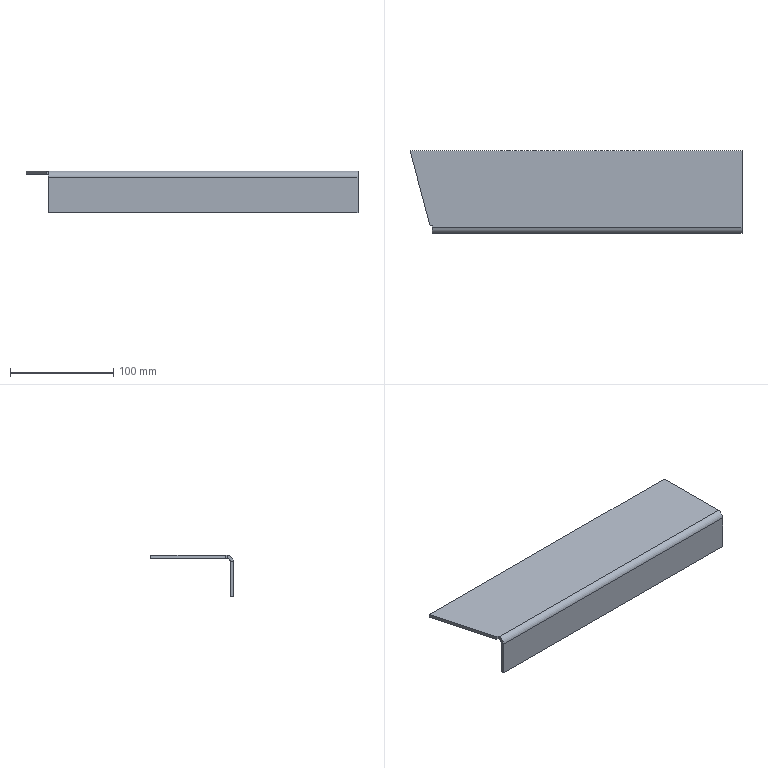Part | SolidWorks | features EdgeFlange 1, FlatPattern 1, ICE 1, SMBaseFlange 1, SheetMetal 1 | 1 solid | 16 faces | box 321.436 x 80 x 40 mm | volume 106111 mm3 | plane 14 | cylinder 2 | commonest cylinder face diameters 6 x1 12 x1
STEP:
#1=CARTESIAN_POINT('',(-2.01,7.5,0.));
#2=VERTEX_POINT('',#1);
#3=CARTESIAN_POINT('',(-2.01,7.5,-3.));
#4=VERTEX_POINT('',#3);
#5=CARTESIAN_POINT('',(-2.01,7.5,-3.));
#6=DIRECTION('',(0.,0.,-1.));
#7=VECTOR('',#6,1000.);
#8=LINE('',#5,#7);
#9=EDGE_CURVE('',#2,#4,#8,.T.);
#10=ORIENTED_EDGE('',*,*,#9,.F.);
#11=CARTESIAN_POINT('',(-21.436,80.,0.));
#12=VERTEX_POINT('',#11);
#13=CARTESIAN_POINT('',(-21.436,80.,0.));
#14=DIRECTION('',(0.2588,-0.9659,0.));
#15=VECTOR('',#14,1000.);
#16=LINE('',#13,#15);
#17=EDGE_CURVE('',#12,#2,#16,.T.);
#18=ORIENTED_EDGE('',*,*,#17,.F.);
#19=CARTESIAN_POINT('',(-21.436,80.,-3.));
#20=VERTEX_POINT('',#19);
#21=CARTESIAN_POINT('',(-21.436,80.,-3.));
#22=DIRECTION('',(0.,0.,1.));
#23=VECTOR('',#22,1000.);
#24=LINE('',#21,#23);
#25=EDGE_CURVE('',#20,#12,#24,.T.);
#26=ORIENTED_EDGE('',*,*,#25,.F.);
#27=CARTESIAN_POINT('',(-21.436,80.,-3.));
#28=DIRECTION('',(0.2588,-0.9659,0.));
#29=VECTOR('',#28,1000.);
#30=LINE('',#27,#29);
#31=EDGE_CURVE('',#20,#4,#30,.T.);
#32=ORIENTED_EDGE('',*,*,#31,.T.);
#33=EDGE_LOOP('',(#10,#18,#26,#32));
#34=FACE_OUTER_BOUND('',#33,.T.);
#35=CARTESIAN_POINT('',(-21.436,80.,-3.));
#36=DIRECTION('',(-0.9659,-0.2588,0.));
#37=DIRECTION('',(0.2588,-0.9659,0.));
#38=AXIS2_PLACEMENT_3D('',#35,#36,#37);
#39=PLANE('',#38);
#40=ADVANCED_FACE('',(#34),#39,.T.);
#41=CARTESIAN_POINT('',(0.,7.5,-3.));
#42=VERTEX_POINT('',#41);
#43=CARTESIAN_POINT('',(-1.5,7.5,-3.));
#44=DIRECTION('',(1.,0.,0.));
#45=VECTOR('',#44,1000.);
#46=LINE('',#43,#45);
#47=EDGE_CURVE('',#4,#42,#46,.T.);
#48=ORIENTED_EDGE('',*,*,#47,.F.);
#49=ORIENTED_EDGE('',*,*,#31,.F.);
#50=CARTESIAN_POINT('',(300.,80.,-3.));
#51=VERTEX_POINT('',#50);
#52=CARTESIAN_POINT('',(300.,80.,-3.));
#53=DIRECTION('',(-1.,0.,0.));
#54=VECTOR('',#53,1000.);
#55=LINE('',#52,#54);
#56=EDGE_CURVE('',#51,#20,#55,.T.);
#57=ORIENTED_EDGE('',*,*,#56,.F.);
#58=CARTESIAN_POINT('',(300.,6.,-3.));
#59=VERTEX_POINT('',#58);
#60=CARTESIAN_POINT('',(300.,0.,-3.));
#61=DIRECTION('',(0.,1.,0.));
#62=VECTOR('',#61,1000.);
#63=LINE('',#60,#62);
#64=EDGE_CURVE('',#59,#51,#63,.T.);
#65=ORIENTED_EDGE('',*,*,#64,.F.);
#66=CARTESIAN_POINT('',(0.,6.,-3.));
#67=VERTEX_POINT('',#66);
#68=CARTESIAN_POINT('',(0.,6.,-3.));
#69=DIRECTION('',(1.,0.,0.));
#70=VECTOR('',#69,1000.);
#71=LINE('',#68,#70);
#72=EDGE_CURVE('',#67,#59,#71,.T.);
#73=ORIENTED_EDGE('',*,*,#72,.F.);
#74=CARTESIAN_POINT('',(0.,7.5,-3.));
#75=DIRECTION('',(0.,-1.,0.));
#76=VECTOR('',#75,1000.);
#77=LINE('',#74,#76);
#78=EDGE_CURVE('',#42,#67,#77,.T.);
#79=ORIENTED_EDGE('',*,*,#78,.F.);
#80=EDGE_LOOP('',(#48,#49,#57,#65,#73,#79));
#81=FACE_OUTER_BOUND('',#80,.T.);
#82=CARTESIAN_POINT('',(0.,0.,-3.));
#83=DIRECTION('',(0.,0.,1.));
#84=DIRECTION('',(1.,0.,0.));
#85=AXIS2_PLACEMENT_3D('',#82,#83,#84);
#86=PLANE('',#85);
#87=ADVANCED_FACE('',(#81),#86,.F.);
#88=ORIENTED_EDGE('',*,*,#17,.T.);
#89=CARTESIAN_POINT('',(0.,7.5,0.));
#90=VERTEX_POINT('',#89);
#91=CARTESIAN_POINT('',(0.,7.5,0.));
#92=DIRECTION('',(1.,0.,0.));
#93=VECTOR('',#92,1000.);
#94=LINE('',#91,#93);
#95=EDGE_CURVE('',#2,#90,#94,.T.);
#96=ORIENTED_EDGE('',*,*,#95,.T.);
#97=CARTESIAN_POINT('',(0.,6.,0.));
#98=VERTEX_POINT('',#97);
#99=CARTESIAN_POINT('',(0.,0.,0.));
#100=DIRECTION('',(0.,-1.,0.));
#101=VECTOR('',#100,1000.);
#102=LINE('',#99,#101);
#103=EDGE_CURVE('',#90,#98,#102,.T.);
#104=ORIENTED_EDGE('',*,*,#103,.T.);
#105=CARTESIAN_POINT('',(300.,6.,0.));
#106=VERTEX_POINT('',#105);
#107=CARTESIAN_POINT('',(0.,6.,0.));
#108=DIRECTION('',(1.,0.,0.));
#109=VECTOR('',#108,1000.);
#110=LINE('',#107,#109);
#111=EDGE_CURVE('',#98,#106,#110,.T.);
#112=ORIENTED_EDGE('',*,*,#111,.T.);
#113=CARTESIAN_POINT('',(300.,80.,0.));
#114=VERTEX_POINT('',#113);
#115=CARTESIAN_POINT('',(300.,0.,0.));
#116=DIRECTION('',(0.,1.,0.));
#117=VECTOR('',#116,1000.);
#118=LINE('',#115,#117);
#119=EDGE_CURVE('',#106,#114,#118,.T.);
#120=ORIENTED_EDGE('',*,*,#119,.T.);
#121=CARTESIAN_POINT('',(300.,80.,0.));
#122=DIRECTION('',(-1.,0.,0.));
#123=VECTOR('',#122,1000.);
#124=LINE('',#121,#123);
#125=EDGE_CURVE('',#114,#12,#124,.T.);
#126=ORIENTED_EDGE('',*,*,#125,.T.);
#127=EDGE_LOOP('',(#88,#96,#104,#112,#120,#126));
#128=FACE_OUTER_BOUND('',#127,.T.);
#129=CARTESIAN_POINT('',(0.,0.,0.));
#130=DIRECTION('',(0.,0.,1.));
#131=DIRECTION('',(1.,0.,0.));
#132=AXIS2_PLACEMENT_3D('',#129,#130,#131);
#133=PLANE('',#132);
#134=ADVANCED_FACE('',(#128),#133,.T.);
#135=CARTESIAN_POINT('',(300.,6.,-3.));
#136=DIRECTION('',(0.,0.,1.));
#137=VECTOR('',#136,1000.);
#138=LINE('',#135,#137);
#139=EDGE_CURVE('',#59,#106,#138,.T.);
#140=ORIENTED_EDGE('',*,*,#139,.F.);
#141=ORIENTED_EDGE('',*,*,#64,.T.);
#142=CARTESIAN_POINT('',(300.,80.,-3.));
#143=DIRECTION('',(0.,0.,1.));
#144=VECTOR('',#143,1000.);
#145=LINE('',#142,#144);
#146=EDGE_CURVE('',#51,#114,#145,.T.);
#147=ORIENTED_EDGE('',*,*,#146,.T.);
#148=ORIENTED_EDGE('',*,*,#119,.F.);
#149=EDGE_LOOP('',(#140,#141,#147,#148));
#150=FACE_OUTER_BOUND('',#149,.T.);
#151=CARTESIAN_POINT('',(300.,0.,-3.));
#152=DIRECTION('',(1.,0.,0.));
#153=DIRECTION('',(0.,0.,-1.));
#154=AXIS2_PLACEMENT_3D('',#151,#152,#153);
#155=PLANE('',#154);
#156=ADVANCED_FACE('',(#150),#155,.T.);
#157=ORIENTED_EDGE('',*,*,#125,.F.);
#158=ORIENTED_EDGE('',*,*,#146,.F.);
#159=ORIENTED_EDGE('',*,*,#56,.T.);
#160=ORIENTED_EDGE('',*,*,#25,.T.);
#161=EDGE_LOOP('',(#157,#158,#159,#160));
#162=FACE_OUTER_BOUND('',#161,.T.);
#163=CARTESIAN_POINT('',(300.,80.,-3.));
#164=DIRECTION('',(0.,1.,0.));
#165=DIRECTION('',(-1.,0.,0.));
#166=AXIS2_PLACEMENT_3D('',#163,#164,#165);
#167=PLANE('',#166);
#168=ADVANCED_FACE('',(#162),#167,.T.);
#169=ORIENTED_EDGE('',*,*,#95,.F.);
#170=ORIENTED_EDGE('',*,*,#9,.T.);
#171=ORIENTED_EDGE('',*,*,#47,.T.);
#172=CARTESIAN_POINT('',(0.,7.5,-3.));
#173=DIRECTION('',(0.,0.,1.));
#174=VECTOR('',#173,1000.);
#175=LINE('',#172,#174);
#176=EDGE_CURVE('',#42,#90,#175,.T.);
#177=ORIENTED_EDGE('',*,*,#176,.T.);
#178=EDGE_LOOP('',(#169,#170,#171,#177));
#179=FACE_OUTER_BOUND('',#178,.T.);
#180=CARTESIAN_POINT('',(-1.5,7.5,-3.));
#181=DIRECTION('',(0.,-1.,0.));
#182=DIRECTION('',(0.,0.,-1.));
#183=AXIS2_PLACEMENT_3D('',#180,#181,#182);
#184=PLANE('',#183);
#185=ADVANCED_FACE('',(#179),#184,.T.);
#186=ORIENTED_EDGE('',*,*,#103,.F.);
#187=ORIENTED_EDGE('',*,*,#176,.F.);
#188=ORIENTED_EDGE('',*,*,#78,.T.);
#189=CARTESIAN_POINT('',(0.,6.,-3.));
#190=DIRECTION('',(0.,0.,1.));
#191=VECTOR('',#190,1000.);
#192=LINE('',#189,#191);
#193=EDGE_CURVE('',#67,#98,#192,.T.);
#194=ORIENTED_EDGE('',*,*,#193,.T.);
#195=EDGE_LOOP('',(#186,#187,#188,#194));
#196=FACE_OUTER_BOUND('',#195,.T.);
#197=CARTESIAN_POINT('',(0.,7.5,-3.));
#198=DIRECTION('',(-1.,0.,0.));
#199=DIRECTION('',(0.,0.,1.));
#200=AXIS2_PLACEMENT_3D('',#197,#198,#199);
#201=PLANE('',#200);
#202=ADVANCED_FACE('',(#196),#201,.T.);
#203=CARTESIAN_POINT('',(300.,3.,-6.));
#204=VERTEX_POINT('',#203);
#205=CARTESIAN_POINT('',(300.,0.,-6.));
#206=VERTEX_POINT('',#205);
#207=CARTESIAN_POINT('',(300.,0.,-6.));
#208=DIRECTION('',(0.,-1.,0.));
#209=VECTOR('',#208,1000.);
#210=LINE('',#207,#209);
#211=EDGE_CURVE('',#204,#206,#210,.T.);
#212=ORIENTED_EDGE('',*,*,#211,.F.);
#213=CARTESIAN_POINT('',(300.,6.,-6.));
#214=DIRECTION('',(1.,0.,0.));
#215=DIRECTION('',(0.,0.,1.));
#216=AXIS2_PLACEMENT_3D('',#213,#214,#215);
#217=CIRCLE('',#216,3.);
#218=EDGE_CURVE('',#59,#204,#217,.T.);
#219=ORIENTED_EDGE('',*,*,#218,.F.);
#220=ORIENTED_EDGE('',*,*,#139,.T.);
#221=CARTESIAN_POINT('',(300.,6.,-6.));
#222=DIRECTION('',(1.,0.,0.));
#223=DIRECTION('',(0.,0.,1.));
#224=AXIS2_PLACEMENT_3D('',#221,#222,#223);
#225=CIRCLE('',#224,6.);
#226=EDGE_CURVE('',#106,#206,#225,.T.);
#227=ORIENTED_EDGE('',*,*,#226,.T.);
#228=EDGE_LOOP('',(#212,#219,#220,#227));
#229=FACE_OUTER_BOUND('',#228,.T.);
#230=CARTESIAN_POINT('',(300.,6.,-6.));
#231=DIRECTION('',(1.,0.,0.));
#232=DIRECTION('',(0.,0.,-1.));
#233=AXIS2_PLACEMENT_3D('',#230,#231,#232);
#234=PLANE('',#233);
#235=ADVANCED_FACE('',(#229),#234,.T.);
#236=CARTESIAN_POINT('',(0.,3.,-6.));
#237=VERTEX_POINT('',#236);
#238=CARTESIAN_POINT('',(0.,6.,-6.));
#239=DIRECTION('',(-1.,0.,0.));
#240=DIRECTION('',(0.,0.,1.));
#241=AXIS2_PLACEMENT_3D('',#238,#239,#240);
#242=CIRCLE('',#241,3.);
#243=EDGE_CURVE('',#237,#67,#242,.T.);
#244=ORIENTED_EDGE('',*,*,#243,.F.);
#245=CARTESIAN_POINT('',(0.,0.,-6.));
#246=VERTEX_POINT('',#245);
#247=CARTESIAN_POINT('',(0.,3.,-6.));
#248=DIRECTION('',(0.,-1.,0.));
#249=VECTOR('',#248,1000.);
#250=LINE('',#247,#249);
#251=EDGE_CURVE('',#237,#246,#250,.T.);
#252=ORIENTED_EDGE('',*,*,#251,.T.);
#253=CARTESIAN_POINT('',(0.,6.,-6.));
#254=DIRECTION('',(-1.,0.,0.));
#255=DIRECTION('',(0.,0.,1.));
#256=AXIS2_PLACEMENT_3D('',#253,#254,#255);
#257=CIRCLE('',#256,6.);
#258=EDGE_CURVE('',#246,#98,#257,.T.);
#259=ORIENTED_EDGE('',*,*,#258,.T.);
#260=ORIENTED_EDGE('',*,*,#193,.F.);
#261=EDGE_LOOP('',(#244,#252,#259,#260));
#262=FACE_OUTER_BOUND('',#261,.T.);
#263=CARTESIAN_POINT('',(0.,6.,-6.));
#264=DIRECTION('',(1.,0.,0.));
#265=DIRECTION('',(0.,0.,-1.));
#266=AXIS2_PLACEMENT_3D('',#263,#264,#265);
#267=PLANE('',#266);
#268=ADVANCED_FACE('',(#262),#267,.F.);
#269=ORIENTED_EDGE('',*,*,#111,.F.);
#270=ORIENTED_EDGE('',*,*,#258,.F.);
#271=CARTESIAN_POINT('',(300.,0.,-6.));
#272=DIRECTION('',(1.,0.,0.));
#273=VECTOR('',#272,1000.);
#274=LINE('',#271,#273);
#275=EDGE_CURVE('',#246,#206,#274,.T.);
#276=ORIENTED_EDGE('',*,*,#275,.T.);
#277=ORIENTED_EDGE('',*,*,#226,.F.);
#278=EDGE_LOOP('',(#269,#270,#276,#277));
#279=FACE_OUTER_BOUND('',#278,.T.);
#280=CARTESIAN_POINT('',(0.,6.,-6.));
#281=DIRECTION('',(-1.,0.,0.));
#282=DIRECTION('',(0.,-1.,0.));
#283=AXIS2_PLACEMENT_3D('',#280,#281,#282);
#284=CYLINDRICAL_SURFACE('',#283,6.);
#285=ADVANCED_FACE('',(#279),#284,.T.);
#286=ORIENTED_EDGE('',*,*,#72,.T.);
#287=ORIENTED_EDGE('',*,*,#218,.T.);
#288=CARTESIAN_POINT('',(300.,3.,-6.));
#289=DIRECTION('',(-1.,0.,0.));
#290=VECTOR('',#289,1000.);
#291=LINE('',#288,#290);
#292=EDGE_CURVE('',#204,#237,#291,.T.);
#293=ORIENTED_EDGE('',*,*,#292,.T.);
#294=ORIENTED_EDGE('',*,*,#243,.T.);
#295=EDGE_LOOP('',(#286,#287,#293,#294));
#296=FACE_OUTER_BOUND('',#295,.T.);
#297=CARTESIAN_POINT('',(0.,6.,-6.));
#298=DIRECTION('',(-1.,0.,0.));
#299=DIRECTION('',(0.,-1.,0.));
#300=AXIS2_PLACEMENT_3D('',#297,#298,#299);
#301=CYLINDRICAL_SURFACE('',#300,3.);
#302=ADVANCED_FACE('',(#296),#301,.F.);
#303=ORIENTED_EDGE('',*,*,#251,.F.);
#304=CARTESIAN_POINT('',(0.,3.,-40.));
#305=VERTEX_POINT('',#304);
#306=CARTESIAN_POINT('',(0.,3.,-40.));
#307=DIRECTION('',(0.,0.,-1.));
#308=VECTOR('',#307,1000.);
#309=LINE('',#306,#308);
#310=EDGE_CURVE('',#237,#305,#309,.T.);
#311=ORIENTED_EDGE('',*,*,#310,.T.);
#312=CARTESIAN_POINT('',(0.,0.,-40.));
#313=VERTEX_POINT('',#312);
#314=CARTESIAN_POINT('',(0.,0.,-40.));
#315=DIRECTION('',(0.,1.,0.));
#316=VECTOR('',#315,1000.);
#317=LINE('',#314,#316);
#318=EDGE_CURVE('',#313,#305,#317,.T.);
#319=ORIENTED_EDGE('',*,*,#318,.F.);
#320=CARTESIAN_POINT('',(0.,0.,0.));
#321=DIRECTION('',(0.,0.,-1.));
#322=VECTOR('',#321,1000.);
#323=LINE('',#320,#322);
#324=EDGE_CURVE('',#246,#313,#323,.T.);
#325=ORIENTED_EDGE('',*,*,#324,.F.);
#326=EDGE_LOOP('',(#303,#311,#319,#325));
#327=FACE_OUTER_BOUND('',#326,.T.);
#328=CARTESIAN_POINT('',(0.,0.,-40.));
#329=DIRECTION('',(1.,0.,0.));
#330=DIRECTION('',(0.,0.,-1.));
#331=AXIS2_PLACEMENT_3D('',#328,#329,#330);
#332=PLANE('',#331);
#333=ADVANCED_FACE('',(#327),#332,.F.);
#334=ORIENTED_EDGE('',*,*,#211,.T.);
#335=CARTESIAN_POINT('',(300.,0.,-40.));
#336=VERTEX_POINT('',#335);
#337=CARTESIAN_POINT('',(300.,0.,0.));
#338=DIRECTION('',(0.,0.,1.));
#339=VECTOR('',#338,1000.);
#340=LINE('',#337,#339);
#341=EDGE_CURVE('',#336,#206,#340,.T.);
#342=ORIENTED_EDGE('',*,*,#341,.F.);
#343=CARTESIAN_POINT('',(300.,3.,-40.));
#344=VERTEX_POINT('',#343);
#345=CARTESIAN_POINT('',(300.,0.,-40.));
#346=DIRECTION('',(0.,1.,0.));
#347=VECTOR('',#346,1000.);
#348=LINE('',#345,#347);
#349=EDGE_CURVE('',#336,#344,#348,.T.);
#350=ORIENTED_EDGE('',*,*,#349,.T.);
#351=CARTESIAN_POINT('',(300.,3.,-3.));
#352=DIRECTION('',(0.,0.,1.));
#353=VECTOR('',#352,1000.);
#354=LINE('',#351,#353);
#355=EDGE_CURVE('',#344,#204,#354,.T.);
#356=ORIENTED_EDGE('',*,*,#355,.T.);
#357=EDGE_LOOP('',(#334,#342,#350,#356));
#358=FACE_OUTER_BOUND('',#357,.T.);
#359=CARTESIAN_POINT('',(300.,0.,-3.));
#360=DIRECTION('',(-1.,0.,0.));
#361=DIRECTION('',(0.,0.,1.));
#362=AXIS2_PLACEMENT_3D('',#359,#360,#361);
#363=PLANE('',#362);
#364=ADVANCED_FACE('',(#358),#363,.F.);
#365=ORIENTED_EDGE('',*,*,#275,.F.);
#366=ORIENTED_EDGE('',*,*,#324,.T.);
#367=CARTESIAN_POINT('',(0.,0.,-40.));
#368=DIRECTION('',(1.,0.,0.));
#369=VECTOR('',#368,1000.);
#370=LINE('',#367,#369);
#371=EDGE_CURVE('',#313,#336,#370,.T.);
#372=ORIENTED_EDGE('',*,*,#371,.T.);
#373=ORIENTED_EDGE('',*,*,#341,.T.);
#374=EDGE_LOOP('',(#365,#366,#372,#373));
#375=FACE_OUTER_BOUND('',#374,.T.);
#376=CARTESIAN_POINT('',(0.,0.,0.));
#377=DIRECTION('',(0.,1.,0.));
#378=DIRECTION('',(0.,0.,1.));
#379=AXIS2_PLACEMENT_3D('',#376,#377,#378);
#380=PLANE('',#379);
#381=ADVANCED_FACE('',(#375),#380,.F.);
#382=ORIENTED_EDGE('',*,*,#310,.F.);
#383=ORIENTED_EDGE('',*,*,#292,.F.);
#384=ORIENTED_EDGE('',*,*,#355,.F.);
#385=CARTESIAN_POINT('',(300.,3.,-40.));
#386=DIRECTION('',(1.,0.,0.));
#387=VECTOR('',#386,1000.);
#388=LINE('',#385,#387);
#389=EDGE_CURVE('',#305,#344,#388,.T.);
#390=ORIENTED_EDGE('',*,*,#389,.F.);
#391=EDGE_LOOP('',(#382,#383,#384,#390));
#392=FACE_OUTER_BOUND('',#391,.T.);
#393=CARTESIAN_POINT('',(0.,3.,0.));
#394=DIRECTION('',(0.,1.,0.));
#395=DIRECTION('',(0.,0.,1.));
#396=AXIS2_PLACEMENT_3D('',#393,#394,#395);
#397=PLANE('',#396);
#398=ADVANCED_FACE('',(#392),#397,.T.);
#399=ORIENTED_EDGE('',*,*,#389,.T.);
#400=ORIENTED_EDGE('',*,*,#349,.F.);
#401=ORIENTED_EDGE('',*,*,#371,.F.);
#402=ORIENTED_EDGE('',*,*,#318,.T.);
#403=EDGE_LOOP('',(#399,#400,#401,#402));
#404=FACE_OUTER_BOUND('',#403,.T.);
#405=CARTESIAN_POINT('',(300.,0.,-40.));
#406=DIRECTION('',(0.,0.,1.));
#407=DIRECTION('',(0.,-1.,0.));
#408=AXIS2_PLACEMENT_3D('',#405,#406,#407);
#409=PLANE('',#408);
#410=ADVANCED_FACE('',(#404),#409,.F.);
#411=CLOSED_SHELL('',(#40,#87,#134,#156,#168,#185,#202,#235,#268,#285,#302,#333,#364,#381,#398,#410));
#412=MANIFOLD_SOLID_BREP('',#411);
#413=CARTESIAN_POINT('',(0.,0.,0.));
#414=DIRECTION('',(0.,0.,1.));
#415=DIRECTION('',(1.,0.,0.));
#416=AXIS2_PLACEMENT_3D('',#413,#414,#415);
#417=(LENGTH_UNIT()NAMED_UNIT(*)SI_UNIT(.MILLI.,.METRE.));
#418=UNCERTAINTY_MEASURE_WITH_UNIT(LENGTH_MEASURE(0.00001),#417,'','');
#419=(NAMED_UNIT(*)PLANE_ANGLE_UNIT()SI_UNIT($,.RADIAN.));
#420=(NAMED_UNIT(*)SI_UNIT($,.STERADIAN.)SOLID_ANGLE_UNIT());
#421=(GEOMETRIC_REPRESENTATION_CONTEXT(3)GLOBAL_UNCERTAINTY_ASSIGNED_CONTEXT((#418))GLOBAL_UNIT_ASSIGNED_CONTEXT((#417,#419,#420))REPRESENTATION_CONTEXT('',''));
#422=ADVANCED_BREP_SHAPE_REPRESENTATION('',(#412,#416),#421);